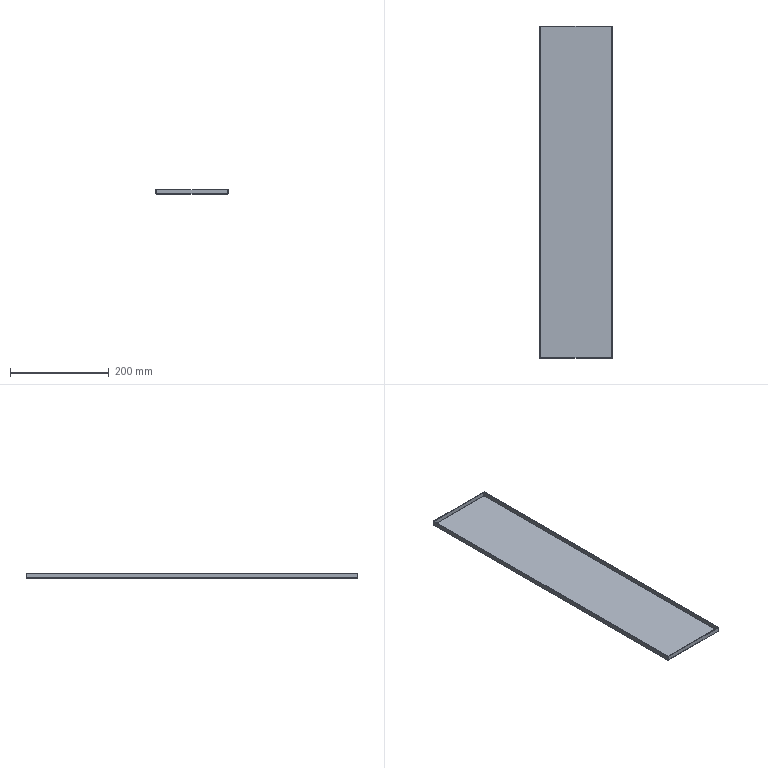Part | SolidWorks | features BaseBody 1 | 1 solid | 38 faces | box 146 x 672 x 10 mm | volume 166908 mm3 | plane 30 | cylinder 8 | commonest cylinder face diameters 0.4 x4 3.4 x4
STEP:
#1=CARTESIAN_POINT('',(1309.,40.5,426.7));
#2=VERTEX_POINT('',#1);
#3=CARTESIAN_POINT('',(1309.,40.7,426.5));
#4=VERTEX_POINT('',#3);
#5=CARTESIAN_POINT('',(1309.,40.7,426.7));
#6=DIRECTION('',(1.,0.,0.));
#7=DIRECTION('',(0.,1.,0.));
#8=AXIS2_PLACEMENT_3D('',#5,#6,#7);
#9=CIRCLE('',#8,0.2);
#10=EDGE_CURVE('',#2,#4,#9,.T.);
#11=ORIENTED_EDGE('',*,*,#10,.F.);
#12=CARTESIAN_POINT('',(1451.,40.5,426.7));
#13=VERTEX_POINT('',#12);
#14=CARTESIAN_POINT('',(1309.,40.5,426.7));
#15=DIRECTION('',(-1.,0.,0.));
#16=VECTOR('',#15,1000.);
#17=LINE('',#14,#16);
#18=EDGE_CURVE('',#13,#2,#17,.T.);
#19=ORIENTED_EDGE('',*,*,#18,.F.);
#20=CARTESIAN_POINT('',(1451.,40.7,426.5));
#21=VERTEX_POINT('',#20);
#22=CARTESIAN_POINT('',(1451.,40.7,426.7));
#23=DIRECTION('',(-1.,0.,0.));
#24=DIRECTION('',(0.,1.,0.));
#25=AXIS2_PLACEMENT_3D('',#22,#23,#24);
#26=CIRCLE('',#25,0.2);
#27=EDGE_CURVE('',#21,#13,#26,.T.);
#28=ORIENTED_EDGE('',*,*,#27,.F.);
#29=CARTESIAN_POINT('',(1309.,40.7,426.5));
#30=DIRECTION('',(1.,0.,0.));
#31=VECTOR('',#30,1000.);
#32=LINE('',#29,#31);
#33=EDGE_CURVE('',#4,#21,#32,.T.);
#34=ORIENTED_EDGE('',*,*,#33,.F.);
#35=EDGE_LOOP('',(#11,#19,#28,#34));
#36=FACE_OUTER_BOUND('',#35,.T.);
#37=CARTESIAN_POINT('',(613.969,40.7,426.7));
#38=DIRECTION('',(1.,0.,0.));
#39=DIRECTION('',(0.,1.,0.));
#40=AXIS2_PLACEMENT_3D('',#37,#38,#39);
#41=CYLINDRICAL_SURFACE('',#40,0.2);
#42=ADVANCED_FACE('',(#36),#41,.F.);
#43=CARTESIAN_POINT('',(1309.,39.,426.7));
#44=VERTEX_POINT('',#43);
#45=CARTESIAN_POINT('',(1309.,40.7,425.));
#46=VERTEX_POINT('',#45);
#47=CARTESIAN_POINT('',(1309.,40.7,426.7));
#48=DIRECTION('',(1.,0.,0.));
#49=DIRECTION('',(0.,1.,0.));
#50=AXIS2_PLACEMENT_3D('',#47,#48,#49);
#51=CIRCLE('',#50,1.7);
#52=EDGE_CURVE('',#44,#46,#51,.T.);
#53=ORIENTED_EDGE('',*,*,#52,.T.);
#54=CARTESIAN_POINT('',(1451.,40.7,425.));
#55=VERTEX_POINT('',#54);
#56=CARTESIAN_POINT('',(1309.,40.7,425.));
#57=DIRECTION('',(1.,0.,0.));
#58=VECTOR('',#57,1000.);
#59=LINE('',#56,#58);
#60=EDGE_CURVE('',#46,#55,#59,.T.);
#61=ORIENTED_EDGE('',*,*,#60,.T.);
#62=CARTESIAN_POINT('',(1451.,39.,426.7));
#63=VERTEX_POINT('',#62);
#64=CARTESIAN_POINT('',(1451.,40.7,426.7));
#65=DIRECTION('',(-1.,0.,0.));
#66=DIRECTION('',(0.,1.,0.));
#67=AXIS2_PLACEMENT_3D('',#64,#65,#66);
#68=CIRCLE('',#67,1.7);
#69=EDGE_CURVE('',#55,#63,#68,.T.);
#70=ORIENTED_EDGE('',*,*,#69,.T.);
#71=CARTESIAN_POINT('',(1309.,39.,426.7));
#72=DIRECTION('',(-1.,0.,0.));
#73=VECTOR('',#72,1000.);
#74=LINE('',#71,#73);
#75=EDGE_CURVE('',#63,#44,#74,.T.);
#76=ORIENTED_EDGE('',*,*,#75,.T.);
#77=EDGE_LOOP('',(#53,#61,#70,#76));
#78=FACE_OUTER_BOUND('',#77,.T.);
#79=CARTESIAN_POINT('',(613.969,40.7,426.7));
#80=DIRECTION('',(1.,0.,0.));
#81=DIRECTION('',(0.,1.,0.));
#82=AXIS2_PLACEMENT_3D('',#79,#80,#81);
#83=CYLINDRICAL_SURFACE('',#82,1.7);
#84=ADVANCED_FACE('',(#78),#83,.T.);
#85=CARTESIAN_POINT('',(1308.5,709.,426.7));
#86=VERTEX_POINT('',#85);
#87=CARTESIAN_POINT('',(1308.7,709.,426.5));
#88=VERTEX_POINT('',#87);
#89=CARTESIAN_POINT('',(1308.7,709.,426.7));
#90=DIRECTION('',(0.,-1.,0.));
#91=DIRECTION('',(0.,0.,-1.));
#92=AXIS2_PLACEMENT_3D('',#89,#90,#91);
#93=CIRCLE('',#92,0.2);
#94=EDGE_CURVE('',#86,#88,#93,.T.);
#95=ORIENTED_EDGE('',*,*,#94,.F.);
#96=CARTESIAN_POINT('',(1308.5,41.,426.7));
#97=VERTEX_POINT('',#96);
#98=CARTESIAN_POINT('',(1308.5,709.,426.7));
#99=DIRECTION('',(0.,1.,0.));
#100=VECTOR('',#99,1000.);
#101=LINE('',#98,#100);
#102=EDGE_CURVE('',#97,#86,#101,.T.);
#103=ORIENTED_EDGE('',*,*,#102,.F.);
#104=CARTESIAN_POINT('',(1308.7,41.,426.5));
#105=VERTEX_POINT('',#104);
#106=CARTESIAN_POINT('',(1308.7,41.,426.7));
#107=DIRECTION('',(0.,1.,0.));
#108=DIRECTION('',(0.,0.,-1.));
#109=AXIS2_PLACEMENT_3D('',#106,#107,#108);
#110=CIRCLE('',#109,0.2);
#111=EDGE_CURVE('',#105,#97,#110,.T.);
#112=ORIENTED_EDGE('',*,*,#111,.F.);
#113=CARTESIAN_POINT('',(1308.7,709.,426.5));
#114=DIRECTION('',(0.,-1.,0.));
#115=VECTOR('',#114,1000.);
#116=LINE('',#113,#115);
#117=EDGE_CURVE('',#88,#105,#116,.T.);
#118=ORIENTED_EDGE('',*,*,#117,.F.);
#119=EDGE_LOOP('',(#95,#103,#112,#118));
#120=FACE_OUTER_BOUND('',#119,.T.);
#121=CARTESIAN_POINT('',(1308.7,1405.634,426.7));
#122=DIRECTION('',(0.,-1.,0.));
#123=DIRECTION('',(0.,0.,-1.));
#124=AXIS2_PLACEMENT_3D('',#121,#122,#123);
#125=CYLINDRICAL_SURFACE('',#124,0.2);
#126=ADVANCED_FACE('',(#120),#125,.F.);
#127=CARTESIAN_POINT('',(1307.,709.,426.7));
#128=VERTEX_POINT('',#127);
#129=CARTESIAN_POINT('',(1308.7,709.,425.));
#130=VERTEX_POINT('',#129);
#131=CARTESIAN_POINT('',(1308.7,709.,426.7));
#132=DIRECTION('',(0.,-1.,0.));
#133=DIRECTION('',(0.,0.,-1.));
#134=AXIS2_PLACEMENT_3D('',#131,#132,#133);
#135=CIRCLE('',#134,1.7);
#136=EDGE_CURVE('',#128,#130,#135,.T.);
#137=ORIENTED_EDGE('',*,*,#136,.T.);
#138=CARTESIAN_POINT('',(1308.7,41.,425.));
#139=VERTEX_POINT('',#138);
#140=CARTESIAN_POINT('',(1308.7,709.,425.));
#141=DIRECTION('',(0.,-1.,0.));
#142=VECTOR('',#141,1000.);
#143=LINE('',#140,#142);
#144=EDGE_CURVE('',#130,#139,#143,.T.);
#145=ORIENTED_EDGE('',*,*,#144,.T.);
#146=CARTESIAN_POINT('',(1307.,41.,426.7));
#147=VERTEX_POINT('',#146);
#148=CARTESIAN_POINT('',(1308.7,41.,426.7));
#149=DIRECTION('',(0.,1.,0.));
#150=DIRECTION('',(0.,0.,-1.));
#151=AXIS2_PLACEMENT_3D('',#148,#149,#150);
#152=CIRCLE('',#151,1.7);
#153=EDGE_CURVE('',#139,#147,#152,.T.);
#154=ORIENTED_EDGE('',*,*,#153,.T.);
#155=CARTESIAN_POINT('',(1307.,709.,426.7));
#156=DIRECTION('',(0.,1.,0.));
#157=VECTOR('',#156,1000.);
#158=LINE('',#155,#157);
#159=EDGE_CURVE('',#147,#128,#158,.T.);
#160=ORIENTED_EDGE('',*,*,#159,.T.);
#161=EDGE_LOOP('',(#137,#145,#154,#160));
#162=FACE_OUTER_BOUND('',#161,.T.);
#163=CARTESIAN_POINT('',(1308.7,1405.634,426.7));
#164=DIRECTION('',(0.,-1.,0.));
#165=DIRECTION('',(0.,0.,-1.));
#166=AXIS2_PLACEMENT_3D('',#163,#164,#165);
#167=CYLINDRICAL_SURFACE('',#166,1.7);
#168=ADVANCED_FACE('',(#162),#167,.T.);
#169=CARTESIAN_POINT('',(1451.,709.5,426.7));
#170=VERTEX_POINT('',#169);
#171=CARTESIAN_POINT('',(1451.,709.3,426.5));
#172=VERTEX_POINT('',#171);
#173=CARTESIAN_POINT('',(1451.,709.3,426.7));
#174=DIRECTION('',(-1.,0.,0.));
#175=DIRECTION('',(0.,0.,1.));
#176=AXIS2_PLACEMENT_3D('',#173,#174,#175);
#177=CIRCLE('',#176,0.2);
#178=EDGE_CURVE('',#170,#172,#177,.T.);
#179=ORIENTED_EDGE('',*,*,#178,.F.);
#180=CARTESIAN_POINT('',(1309.,709.5,426.7));
#181=VERTEX_POINT('',#180);
#182=CARTESIAN_POINT('',(1451.,709.5,426.7));
#183=DIRECTION('',(1.,0.,0.));
#184=VECTOR('',#183,1000.);
#185=LINE('',#182,#184);
#186=EDGE_CURVE('',#181,#170,#185,.T.);
#187=ORIENTED_EDGE('',*,*,#186,.F.);
#188=CARTESIAN_POINT('',(1309.,709.3,426.5));
#189=VERTEX_POINT('',#188);
#190=CARTESIAN_POINT('',(1309.,709.3,426.7));
#191=DIRECTION('',(1.,0.,0.));
#192=DIRECTION('',(0.,0.,1.));
#193=AXIS2_PLACEMENT_3D('',#190,#191,#192);
#194=CIRCLE('',#193,0.2);
#195=EDGE_CURVE('',#189,#181,#194,.T.);
#196=ORIENTED_EDGE('',*,*,#195,.F.);
#197=CARTESIAN_POINT('',(1451.,709.3,426.5));
#198=DIRECTION('',(-1.,0.,0.));
#199=VECTOR('',#198,1000.);
#200=LINE('',#197,#199);
#201=EDGE_CURVE('',#172,#189,#200,.T.);
#202=ORIENTED_EDGE('',*,*,#201,.F.);
#203=EDGE_LOOP('',(#179,#187,#196,#202));
#204=FACE_OUTER_BOUND('',#203,.T.);
#205=CARTESIAN_POINT('',(2154.902,709.3,426.7));
#206=DIRECTION('',(-1.,0.,0.));
#207=DIRECTION('',(0.,0.,1.));
#208=AXIS2_PLACEMENT_3D('',#205,#206,#207);
#209=CYLINDRICAL_SURFACE('',#208,0.2);
#210=ADVANCED_FACE('',(#204),#209,.F.);
#211=CARTESIAN_POINT('',(1451.,711.,426.7));
#212=VERTEX_POINT('',#211);
#213=CARTESIAN_POINT('',(1451.,709.3,425.));
#214=VERTEX_POINT('',#213);
#215=CARTESIAN_POINT('',(1451.,709.3,426.7));
#216=DIRECTION('',(-1.,0.,0.));
#217=DIRECTION('',(0.,0.,1.));
#218=AXIS2_PLACEMENT_3D('',#215,#216,#217);
#219=CIRCLE('',#218,1.7);
#220=EDGE_CURVE('',#212,#214,#219,.T.);
#221=ORIENTED_EDGE('',*,*,#220,.T.);
#222=CARTESIAN_POINT('',(1309.,709.3,425.));
#223=VERTEX_POINT('',#222);
#224=CARTESIAN_POINT('',(1451.,709.3,425.));
#225=DIRECTION('',(-1.,0.,0.));
#226=VECTOR('',#225,1000.);
#227=LINE('',#224,#226);
#228=EDGE_CURVE('',#214,#223,#227,.T.);
#229=ORIENTED_EDGE('',*,*,#228,.T.);
#230=CARTESIAN_POINT('',(1309.,711.,426.7));
#231=VERTEX_POINT('',#230);
#232=CARTESIAN_POINT('',(1309.,709.3,426.7));
#233=DIRECTION('',(1.,0.,0.));
#234=DIRECTION('',(0.,0.,1.));
#235=AXIS2_PLACEMENT_3D('',#232,#233,#234);
#236=CIRCLE('',#235,1.7);
#237=EDGE_CURVE('',#223,#231,#236,.T.);
#238=ORIENTED_EDGE('',*,*,#237,.T.);
#239=CARTESIAN_POINT('',(1451.,711.,426.7));
#240=DIRECTION('',(1.,0.,0.));
#241=VECTOR('',#240,1000.);
#242=LINE('',#239,#241);
#243=EDGE_CURVE('',#231,#212,#242,.T.);
#244=ORIENTED_EDGE('',*,*,#243,.T.);
#245=EDGE_LOOP('',(#221,#229,#238,#244));
#246=FACE_OUTER_BOUND('',#245,.T.);
#247=CARTESIAN_POINT('',(2154.902,709.3,426.7));
#248=DIRECTION('',(-1.,0.,0.));
#249=DIRECTION('',(0.,0.,1.));
#250=AXIS2_PLACEMENT_3D('',#247,#248,#249);
#251=CYLINDRICAL_SURFACE('',#250,1.7);
#252=ADVANCED_FACE('',(#246),#251,.T.);
#253=CARTESIAN_POINT('',(1451.5,41.,426.7));
#254=VERTEX_POINT('',#253);
#255=CARTESIAN_POINT('',(1451.3,41.,426.5));
#256=VERTEX_POINT('',#255);
#257=CARTESIAN_POINT('',(1451.3,41.,426.7));
#258=DIRECTION('',(0.,1.,0.));
#259=DIRECTION('',(0.,0.,1.));
#260=AXIS2_PLACEMENT_3D('',#257,#258,#259);
#261=CIRCLE('',#260,0.2);
#262=EDGE_CURVE('',#254,#256,#261,.T.);
#263=ORIENTED_EDGE('',*,*,#262,.F.);
#264=CARTESIAN_POINT('',(1451.5,709.,426.7));
#265=VERTEX_POINT('',#264);
#266=CARTESIAN_POINT('',(1451.5,41.,426.7));
#267=DIRECTION('',(0.,-1.,0.));
#268=VECTOR('',#267,1000.);
#269=LINE('',#266,#268);
#270=EDGE_CURVE('',#265,#254,#269,.T.);
#271=ORIENTED_EDGE('',*,*,#270,.F.);
#272=CARTESIAN_POINT('',(1451.3,709.,426.5));
#273=VERTEX_POINT('',#272);
#274=CARTESIAN_POINT('',(1451.3,709.,426.7));
#275=DIRECTION('',(0.,-1.,0.));
#276=DIRECTION('',(0.,0.,1.));
#277=AXIS2_PLACEMENT_3D('',#274,#275,#276);
#278=CIRCLE('',#277,0.2);
#279=EDGE_CURVE('',#273,#265,#278,.T.);
#280=ORIENTED_EDGE('',*,*,#279,.F.);
#281=CARTESIAN_POINT('',(1451.3,41.,426.5));
#282=DIRECTION('',(0.,1.,0.));
#283=VECTOR('',#282,1000.);
#284=LINE('',#281,#283);
#285=EDGE_CURVE('',#256,#273,#284,.T.);
#286=ORIENTED_EDGE('',*,*,#285,.F.);
#287=EDGE_LOOP('',(#263,#271,#280,#286));
#288=FACE_OUTER_BOUND('',#287,.T.);
#289=CARTESIAN_POINT('',(1451.3,-664.495,426.7));
#290=DIRECTION('',(0.,1.,0.));
#291=DIRECTION('',(0.,0.,1.));
#292=AXIS2_PLACEMENT_3D('',#289,#290,#291);
#293=CYLINDRICAL_SURFACE('',#292,0.2);
#294=ADVANCED_FACE('',(#288),#293,.F.);
#295=CARTESIAN_POINT('',(1453.,41.,426.7));
#296=VERTEX_POINT('',#295);
#297=CARTESIAN_POINT('',(1451.3,41.,425.));
#298=VERTEX_POINT('',#297);
#299=CARTESIAN_POINT('',(1451.3,41.,426.7));
#300=DIRECTION('',(0.,1.,0.));
#301=DIRECTION('',(0.,0.,1.));
#302=AXIS2_PLACEMENT_3D('',#299,#300,#301);
#303=CIRCLE('',#302,1.7);
#304=EDGE_CURVE('',#296,#298,#303,.T.);
#305=ORIENTED_EDGE('',*,*,#304,.T.);
#306=CARTESIAN_POINT('',(1451.3,709.,425.));
#307=VERTEX_POINT('',#306);
#308=CARTESIAN_POINT('',(1451.3,41.,425.));
#309=DIRECTION('',(0.,1.,0.));
#310=VECTOR('',#309,1000.);
#311=LINE('',#308,#310);
#312=EDGE_CURVE('',#298,#307,#311,.T.);
#313=ORIENTED_EDGE('',*,*,#312,.T.);
#314=CARTESIAN_POINT('',(1453.,709.,426.7));
#315=VERTEX_POINT('',#314);
#316=CARTESIAN_POINT('',(1451.3,709.,426.7));
#317=DIRECTION('',(0.,-1.,0.));
#318=DIRECTION('',(0.,0.,1.));
#319=AXIS2_PLACEMENT_3D('',#316,#317,#318);
#320=CIRCLE('',#319,1.7);
#321=EDGE_CURVE('',#307,#315,#320,.T.);
#322=ORIENTED_EDGE('',*,*,#321,.T.);
#323=CARTESIAN_POINT('',(1453.,41.,426.7));
#324=DIRECTION('',(0.,-1.,0.));
#325=VECTOR('',#324,1000.);
#326=LINE('',#323,#325);
#327=EDGE_CURVE('',#315,#296,#326,.T.);
#328=ORIENTED_EDGE('',*,*,#327,.T.);
#329=EDGE_LOOP('',(#305,#313,#322,#328));
#330=FACE_OUTER_BOUND('',#329,.T.);
#331=CARTESIAN_POINT('',(1451.3,-664.495,426.7));
#332=DIRECTION('',(0.,1.,0.));
#333=DIRECTION('',(0.,0.,1.));
#334=AXIS2_PLACEMENT_3D('',#331,#332,#333);
#335=CYLINDRICAL_SURFACE('',#334,1.7);
#336=ADVANCED_FACE('',(#330),#335,.T.);
#337=CARTESIAN_POINT('',(1451.,41.,426.5));
#338=VERTEX_POINT('',#337);
#339=CARTESIAN_POINT('',(0.,41.,426.5));
#340=DIRECTION('',(1.,0.,0.));
#341=VECTOR('',#340,1000.);
#342=LINE('',#339,#341);
#343=EDGE_CURVE('',#338,#256,#342,.T.);
#344=ORIENTED_EDGE('',*,*,#343,.T.);
#345=ORIENTED_EDGE('',*,*,#285,.T.);
#346=CARTESIAN_POINT('',(1451.,709.,426.5));
#347=VERTEX_POINT('',#346);
#348=CARTESIAN_POINT('',(0.,709.,426.5));
#349=DIRECTION('',(-1.,0.,0.));
#350=VECTOR('',#349,1000.);
#351=LINE('',#348,#350);
#352=EDGE_CURVE('',#273,#347,#351,.T.);
#353=ORIENTED_EDGE('',*,*,#352,.T.);
#354=CARTESIAN_POINT('',(1451.,0.,426.5));
#355=DIRECTION('',(0.,1.,0.));
#356=VECTOR('',#355,1000.);
#357=LINE('',#354,#356);
#358=EDGE_CURVE('',#347,#172,#357,.T.);
#359=ORIENTED_EDGE('',*,*,#358,.T.);
#360=ORIENTED_EDGE('',*,*,#201,.T.);
#361=CARTESIAN_POINT('',(1309.,709.,426.5));
#362=VERTEX_POINT('',#361);
#363=CARTESIAN_POINT('',(1309.,0.,426.5));
#364=DIRECTION('',(0.,-1.,0.));
#365=VECTOR('',#364,1000.);
#366=LINE('',#363,#365);
#367=EDGE_CURVE('',#189,#362,#366,.T.);
#368=ORIENTED_EDGE('',*,*,#367,.T.);
#369=CARTESIAN_POINT('',(0.,709.,426.5));
#370=DIRECTION('',(-1.,0.,0.));
#371=VECTOR('',#370,1000.);
#372=LINE('',#369,#371);
#373=EDGE_CURVE('',#362,#88,#372,.T.);
#374=ORIENTED_EDGE('',*,*,#373,.T.);
#375=ORIENTED_EDGE('',*,*,#117,.T.);
#376=CARTESIAN_POINT('',(1309.,41.,426.5));
#377=VERTEX_POINT('',#376);
#378=CARTESIAN_POINT('',(0.,41.,426.5));
#379=DIRECTION('',(1.,0.,0.));
#380=VECTOR('',#379,1000.);
#381=LINE('',#378,#380);
#382=EDGE_CURVE('',#105,#377,#381,.T.);
#383=ORIENTED_EDGE('',*,*,#382,.T.);
#384=CARTESIAN_POINT('',(1309.,0.,426.5));
#385=DIRECTION('',(0.,-1.,0.));
#386=VECTOR('',#385,1000.);
#387=LINE('',#384,#386);
#388=EDGE_CURVE('',#377,#4,#387,.T.);
#389=ORIENTED_EDGE('',*,*,#388,.T.);
#390=ORIENTED_EDGE('',*,*,#33,.T.);
#391=CARTESIAN_POINT('',(1451.,0.,426.5));
#392=DIRECTION('',(0.,1.,0.));
#393=VECTOR('',#392,1000.);
#394=LINE('',#391,#393);
#395=EDGE_CURVE('',#21,#338,#394,.T.);
#396=ORIENTED_EDGE('',*,*,#395,.T.);
#397=EDGE_LOOP('',(#344,#345,#353,#359,#360,#368,#374,#375,#383,#389,#390,#396));
#398=FACE_OUTER_BOUND('',#397,.T.);
#399=CARTESIAN_POINT('',(0.,0.,426.5));
#400=DIRECTION('',(0.,0.,1.));
#401=DIRECTION('',(1.,0.,0.));
#402=AXIS2_PLACEMENT_3D('',#399,#400,#401);
#403=PLANE('',#402);
#404=ADVANCED_FACE('',(#398),#403,.T.);
#405=ORIENTED_EDGE('',*,*,#382,.F.);
#406=ORIENTED_EDGE('',*,*,#111,.T.);
#407=CARTESIAN_POINT('',(2652.603,41.,426.7));
#408=DIRECTION('',(-1.,0.,0.));
#409=VECTOR('',#408,1000.);
#410=LINE('',#407,#409);
#411=EDGE_CURVE('',#97,#147,#410,.T.);
#412=ORIENTED_EDGE('',*,*,#411,.T.);
#413=ORIENTED_EDGE('',*,*,#153,.F.);
#414=CARTESIAN_POINT('',(1309.,41.,425.));
#415=VERTEX_POINT('',#414);
#416=CARTESIAN_POINT('',(0.,41.,425.));
#417=DIRECTION('',(1.,0.,0.));
#418=VECTOR('',#417,1000.);
#419=LINE('',#416,#418);
#420=EDGE_CURVE('',#139,#415,#419,.T.);
#421=ORIENTED_EDGE('',*,*,#420,.T.);
#422=CARTESIAN_POINT('',(1309.,41.,1793.776));
#423=DIRECTION('',(0.,0.,-1.));
#424=VECTOR('',#423,1000.);
#425=LINE('',#422,#424);
#426=EDGE_CURVE('',#377,#415,#425,.T.);
#427=ORIENTED_EDGE('',*,*,#426,.F.);
#428=EDGE_LOOP('',(#405,#406,#412,#413,#421,#427));
#429=FACE_OUTER_BOUND('',#428,.T.);
#430=CARTESIAN_POINT('',(0.,41.,1793.776));
#431=DIRECTION('',(0.,1.,0.));
#432=DIRECTION('',(1.,0.,0.));
#433=AXIS2_PLACEMENT_3D('',#430,#431,#432);
#434=PLANE('',#433);
#435=ADVANCED_FACE('',(#429),#434,.F.);
#436=CARTESIAN_POINT('',(1309.,709.,425.));
#437=VERTEX_POINT('',#436);
#438=CARTESIAN_POINT('',(1309.,709.,1793.776));
#439=DIRECTION('',(0.,0.,-1.));
#440=VECTOR('',#439,1000.);
#441=LINE('',#438,#440);
#442=EDGE_CURVE('',#362,#437,#441,.T.);
#443=ORIENTED_EDGE('',*,*,#442,.T.);
#444=CARTESIAN_POINT('',(0.,709.,425.));
#445=DIRECTION('',(-1.,0.,0.));
#446=VECTOR('',#445,1000.);
#447=LINE('',#444,#446);
#448=EDGE_CURVE('',#437,#130,#447,.T.);
#449=ORIENTED_EDGE('',*,*,#448,.T.);
#450=ORIENTED_EDGE('',*,*,#136,.F.);
#451=CARTESIAN_POINT('',(2652.603,709.,426.7));
#452=DIRECTION('',(-1.,0.,0.));
#453=VECTOR('',#452,1000.);
#454=LINE('',#451,#453);
#455=EDGE_CURVE('',#86,#128,#454,.T.);
#456=ORIENTED_EDGE('',*,*,#455,.F.);
#457=ORIENTED_EDGE('',*,*,#94,.T.);
#458=ORIENTED_EDGE('',*,*,#373,.F.);
#459=EDGE_LOOP('',(#443,#449,#450,#456,#457,#458));
#460=FACE_OUTER_BOUND('',#459,.T.);
#461=CARTESIAN_POINT('',(0.,709.,1793.776));
#462=DIRECTION('',(0.,-1.,0.));
#463=DIRECTION('',(0.,0.,-1.));
#464=AXIS2_PLACEMENT_3D('',#461,#462,#463);
#465=PLANE('',#464);
#466=ADVANCED_FACE('',(#460),#465,.F.);
#467=ORIENTED_EDGE('',*,*,#352,.F.);
#468=ORIENTED_EDGE('',*,*,#279,.T.);
#469=CARTESIAN_POINT('',(107.397,709.,426.7));
#470=DIRECTION('',(1.,0.,0.));
#471=VECTOR('',#470,1000.);
#472=LINE('',#469,#471);
#473=EDGE_CURVE('',#265,#315,#472,.T.);
#474=ORIENTED_EDGE('',*,*,#473,.T.);
#475=ORIENTED_EDGE('',*,*,#321,.F.);
#476=CARTESIAN_POINT('',(1451.,709.,425.));
#477=VERTEX_POINT('',#476);
#478=CARTESIAN_POINT('',(0.,709.,425.));
#479=DIRECTION('',(-1.,0.,0.));
#480=VECTOR('',#479,1000.);
#481=LINE('',#478,#480);
#482=EDGE_CURVE('',#307,#477,#481,.T.);
#483=ORIENTED_EDGE('',*,*,#482,.T.);
#484=CARTESIAN_POINT('',(1451.,709.,1793.776));
#485=DIRECTION('',(0.,0.,-1.));
#486=VECTOR('',#485,1000.);
#487=LINE('',#484,#486);
#488=EDGE_CURVE('',#347,#477,#487,.T.);
#489=ORIENTED_EDGE('',*,*,#488,.F.);
#490=EDGE_LOOP('',(#467,#468,#474,#475,#483,#489));
#491=FACE_OUTER_BOUND('',#490,.T.);
#492=CARTESIAN_POINT('',(0.,709.,1793.776));
#493=DIRECTION('',(0.,-1.,0.));
#494=DIRECTION('',(0.,0.,-1.));
#495=AXIS2_PLACEMENT_3D('',#492,#493,#494);
#496=PLANE('',#495);
#497=ADVANCED_FACE('',(#491),#496,.F.);
#498=CARTESIAN_POINT('',(1451.,41.,425.));
#499=VERTEX_POINT('',#498);
#500=CARTESIAN_POINT('',(1451.,41.,1793.776));
#501=DIRECTION('',(0.,0.,-1.));
#502=VECTOR('',#501,1000.);
#503=LINE('',#500,#502);
#504=EDGE_CURVE('',#338,#499,#503,.T.);
#505=ORIENTED_EDGE('',*,*,#504,.T.);
#506=CARTESIAN_POINT('',(0.,41.,425.));
#507=DIRECTION('',(1.,0.,0.));
#508=VECTOR('',#507,1000.);
#509=LINE('',#506,#508);
#510=EDGE_CURVE('',#499,#298,#509,.T.);
#511=ORIENTED_EDGE('',*,*,#510,.T.);
#512=ORIENTED_EDGE('',*,*,#304,.F.);
#513=CARTESIAN_POINT('',(107.397,41.,426.7));
#514=DIRECTION('',(1.,0.,0.));
#515=VECTOR('',#514,1000.);
#516=LINE('',#513,#515);
#517=EDGE_CURVE('',#254,#296,#516,.T.);
#518=ORIENTED_EDGE('',*,*,#517,.F.);
#519=ORIENTED_EDGE('',*,*,#262,.T.);
#520=ORIENTED_EDGE('',*,*,#343,.F.);
#521=EDGE_LOOP('',(#505,#511,#512,#518,#519,#520));
#522=FACE_OUTER_BOUND('',#521,.T.);
#523=CARTESIAN_POINT('',(0.,41.,1793.776));
#524=DIRECTION('',(0.,1.,0.));
#525=DIRECTION('',(1.,0.,0.));
#526=AXIS2_PLACEMENT_3D('',#523,#524,#525);
#527=PLANE('',#526);
#528=ADVANCED_FACE('',(#522),#527,.F.);
#529=ORIENTED_EDGE('',*,*,#312,.F.);
#530=ORIENTED_EDGE('',*,*,#510,.F.);
#531=CARTESIAN_POINT('',(1451.,0.,425.));
#532=DIRECTION('',(0.,1.,0.));
#533=VECTOR('',#532,1000.);
#534=LINE('',#531,#533);
#535=EDGE_CURVE('',#55,#499,#534,.T.);
#536=ORIENTED_EDGE('',*,*,#535,.F.);
#537=ORIENTED_EDGE('',*,*,#60,.F.);
#538=CARTESIAN_POINT('',(1309.,0.,425.));
#539=DIRECTION('',(0.,-1.,0.));
#540=VECTOR('',#539,1000.);
#541=LINE('',#538,#540);
#542=EDGE_CURVE('',#415,#46,#541,.T.);
#543=ORIENTED_EDGE('',*,*,#542,.F.);
#544=ORIENTED_EDGE('',*,*,#420,.F.);
#545=ORIENTED_EDGE('',*,*,#144,.F.);
#546=ORIENTED_EDGE('',*,*,#448,.F.);
#547=CARTESIAN_POINT('',(1309.,0.,425.));
#548=DIRECTION('',(0.,-1.,0.));
#549=VECTOR('',#548,1000.);
#550=LINE('',#547,#549);
#551=EDGE_CURVE('',#223,#437,#550,.T.);
#552=ORIENTED_EDGE('',*,*,#551,.F.);
#553=ORIENTED_EDGE('',*,*,#228,.F.);
#554=CARTESIAN_POINT('',(1451.,0.,425.));
#555=DIRECTION('',(0.,1.,0.));
#556=VECTOR('',#555,1000.);
#557=LINE('',#554,#556);
#558=EDGE_CURVE('',#477,#214,#557,.T.);
#559=ORIENTED_EDGE('',*,*,#558,.F.);
#560=ORIENTED_EDGE('',*,*,#482,.F.);
#561=EDGE_LOOP('',(#529,#530,#536,#537,#543,#544,#545,#546,#552,#553,#559,#560));
#562=FACE_OUTER_BOUND('',#561,.T.);
#563=CARTESIAN_POINT('',(0.,0.,425.));
#564=DIRECTION('',(0.,0.,1.));
#565=DIRECTION('',(1.,0.,0.));
#566=AXIS2_PLACEMENT_3D('',#563,#564,#565);
#567=PLANE('',#566);
#568=ADVANCED_FACE('',(#562),#567,.F.);
#569=CARTESIAN_POINT('',(1451.5,39.,435.));
#570=VERTEX_POINT('',#569);
#571=CARTESIAN_POINT('',(1451.5,711.,435.));
#572=VERTEX_POINT('',#571);
#573=CARTESIAN_POINT('',(1451.5,40.5,435.));
#574=DIRECTION('',(0.,1.,0.));
#575=VECTOR('',#574,1000.);
#576=LINE('',#573,#575);
#577=EDGE_CURVE('',#570,#572,#576,.T.);
#578=ORIENTED_EDGE('',*,*,#577,.T.);
#579=CARTESIAN_POINT('',(1451.5,711.,426.7));
#580=VERTEX_POINT('',#579);
#581=CARTESIAN_POINT('',(1451.5,711.,-259.113));
#582=DIRECTION('',(0.,0.,-1.));
#583=VECTOR('',#582,1000.);
#584=LINE('',#581,#583);
#585=EDGE_CURVE('',#572,#580,#584,.T.);
#586=ORIENTED_EDGE('',*,*,#585,.T.);
#587=CARTESIAN_POINT('',(1451.5,711.002,426.7));
#588=DIRECTION('',(0.,-1.,0.));
#589=VECTOR('',#588,1000.);
#590=LINE('',#587,#589);
#591=EDGE_CURVE('',#580,#265,#590,.T.);
#592=ORIENTED_EDGE('',*,*,#591,.T.);
#593=ORIENTED_EDGE('',*,*,#270,.T.);
#594=CARTESIAN_POINT('',(1451.5,39.,426.7));
#595=VERTEX_POINT('',#594);
#596=CARTESIAN_POINT('',(1451.5,38.998,426.7));
#597=DIRECTION('',(0.,1.,0.));
#598=VECTOR('',#597,1000.);
#599=LINE('',#596,#598);
#600=EDGE_CURVE('',#595,#254,#599,.T.);
#601=ORIENTED_EDGE('',*,*,#600,.F.);
#602=CARTESIAN_POINT('',(1451.5,39.,-259.113));
#603=DIRECTION('',(0.,0.,1.));
#604=VECTOR('',#603,1000.);
#605=LINE('',#602,#604);
#606=EDGE_CURVE('',#595,#570,#605,.T.);
#607=ORIENTED_EDGE('',*,*,#606,.T.);
#608=EDGE_LOOP('',(#578,#586,#592,#593,#601,#607));
#609=FACE_OUTER_BOUND('',#608,.T.);
#610=CARTESIAN_POINT('',(1451.5,40.5,-259.113));
#611=DIRECTION('',(1.,0.,0.));
#612=DIRECTION('',(0.,1.,0.));
#613=AXIS2_PLACEMENT_3D('',#610,#611,#612);
#614=PLANE('',#613);
#615=ADVANCED_FACE('',(#609),#614,.F.);
#616=CARTESIAN_POINT('',(1453.,711.,426.7));
#617=VERTEX_POINT('',#616);
#618=CARTESIAN_POINT('',(1453.,711.002,426.7));
#619=DIRECTION('',(0.,-1.,0.));
#620=VECTOR('',#619,1000.);
#621=LINE('',#618,#620);
#622=EDGE_CURVE('',#617,#315,#621,.T.);
#623=ORIENTED_EDGE('',*,*,#622,.T.);
#624=ORIENTED_EDGE('',*,*,#473,.F.);
#625=ORIENTED_EDGE('',*,*,#591,.F.);
#626=CARTESIAN_POINT('',(107.397,711.,426.7));
#627=DIRECTION('',(1.,0.,0.));
#628=VECTOR('',#627,1000.);
#629=LINE('',#626,#628);
#630=EDGE_CURVE('',#580,#617,#629,.T.);
#631=ORIENTED_EDGE('',*,*,#630,.T.);
#632=EDGE_LOOP('',(#623,#624,#625,#631));
#633=FACE_OUTER_BOUND('',#632,.T.);
#634=CARTESIAN_POINT('',(107.397,711.002,426.7));
#635=DIRECTION('',(0.,0.,1.));
#636=DIRECTION('',(1.,0.,0.));
#637=AXIS2_PLACEMENT_3D('',#634,#635,#636);
#638=PLANE('',#637);
#639=ADVANCED_FACE('',(#633),#638,.F.);
#640=ORIENTED_EDGE('',*,*,#327,.F.);
#641=ORIENTED_EDGE('',*,*,#622,.F.);
#642=CARTESIAN_POINT('',(1453.,711.,435.));
#643=VERTEX_POINT('',#642);
#644=CARTESIAN_POINT('',(1453.,711.,-259.113));
#645=DIRECTION('',(0.,0.,1.));
#646=VECTOR('',#645,1000.);
#647=LINE('',#644,#646);
#648=EDGE_CURVE('',#617,#643,#647,.T.);
#649=ORIENTED_EDGE('',*,*,#648,.T.);
#650=CARTESIAN_POINT('',(1453.,39.,435.));
#651=VERTEX_POINT('',#650);
#652=CARTESIAN_POINT('',(1453.,39.,435.));
#653=DIRECTION('',(0.,-1.,0.));
#654=VECTOR('',#653,1000.);
#655=LINE('',#652,#654);
#656=EDGE_CURVE('',#643,#651,#655,.T.);
#657=ORIENTED_EDGE('',*,*,#656,.T.);
#658=CARTESIAN_POINT('',(1453.,39.,426.7));
#659=VERTEX_POINT('',#658);
#660=CARTESIAN_POINT('',(1453.,39.,423.672));
#661=DIRECTION('',(0.,0.,1.));
#662=VECTOR('',#661,1000.);
#663=LINE('',#660,#662);
#664=EDGE_CURVE('',#659,#651,#663,.T.);
#665=ORIENTED_EDGE('',*,*,#664,.F.);
#666=CARTESIAN_POINT('',(1453.,38.998,426.7));
#667=DIRECTION('',(0.,1.,0.));
#668=VECTOR('',#667,1000.);
#669=LINE('',#666,#668);
#670=EDGE_CURVE('',#659,#296,#669,.T.);
#671=ORIENTED_EDGE('',*,*,#670,.T.);
#672=EDGE_LOOP('',(#640,#641,#649,#657,#665,#671));
#673=FACE_OUTER_BOUND('',#672,.T.);
#674=CARTESIAN_POINT('',(1453.,39.,435.));
#675=DIRECTION('',(1.,0.,0.));
#676=DIRECTION('',(0.,1.,0.));
#677=AXIS2_PLACEMENT_3D('',#674,#675,#676);
#678=PLANE('',#677);
#679=ADVANCED_FACE('',(#673),#678,.T.);
#680=ORIENTED_EDGE('',*,*,#517,.T.);
#681=ORIENTED_EDGE('',*,*,#670,.F.);
#682=CARTESIAN_POINT('',(107.397,39.,426.7));
#683=DIRECTION('',(1.,0.,0.));
#684=VECTOR('',#683,1000.);
#685=LINE('',#682,#684);
#686=EDGE_CURVE('',#595,#659,#685,.T.);
#687=ORIENTED_EDGE('',*,*,#686,.F.);
#688=ORIENTED_EDGE('',*,*,#600,.T.);
#689=EDGE_LOOP('',(#680,#681,#687,#688));
#690=FACE_OUTER_BOUND('',#689,.T.);
#691=CARTESIAN_POINT('',(107.397,38.998,426.7));
#692=DIRECTION('',(0.,0.,-1.));
#693=DIRECTION('',(0.,-1.,0.));
#694=AXIS2_PLACEMENT_3D('',#691,#692,#693);
#695=PLANE('',#694);
#696=ADVANCED_FACE('',(#690),#695,.T.);
#697=ORIENTED_EDGE('',*,*,#664,.T.);
#698=CARTESIAN_POINT('',(107.397,39.,435.));
#699=DIRECTION('',(1.,0.,0.));
#700=VECTOR('',#699,1000.);
#701=LINE('',#698,#700);
#702=EDGE_CURVE('',#570,#651,#701,.T.);
#703=ORIENTED_EDGE('',*,*,#702,.F.);
#704=ORIENTED_EDGE('',*,*,#606,.F.);
#705=ORIENTED_EDGE('',*,*,#686,.T.);
#706=EDGE_LOOP('',(#697,#703,#704,#705));
#707=FACE_OUTER_BOUND('',#706,.T.);
#708=CARTESIAN_POINT('',(107.397,39.,-259.113));
#709=DIRECTION('',(0.,1.,0.));
#710=DIRECTION('',(0.,0.,-1.));
#711=AXIS2_PLACEMENT_3D('',#708,#709,#710);
#712=PLANE('',#711);
#713=ADVANCED_FACE('',(#707),#712,.F.);
#714=ORIENTED_EDGE('',*,*,#648,.F.);
#715=ORIENTED_EDGE('',*,*,#630,.F.);
#716=ORIENTED_EDGE('',*,*,#585,.F.);
#717=CARTESIAN_POINT('',(107.397,711.,435.));
#718=DIRECTION('',(1.,0.,0.));
#719=VECTOR('',#718,1000.);
#720=LINE('',#717,#719);
#721=EDGE_CURVE('',#572,#643,#720,.T.);
#722=ORIENTED_EDGE('',*,*,#721,.T.);
#723=EDGE_LOOP('',(#714,#715,#716,#722));
#724=FACE_OUTER_BOUND('',#723,.T.);
#725=CARTESIAN_POINT('',(107.397,711.,-259.113));
#726=DIRECTION('',(0.,-1.,0.));
#727=DIRECTION('',(0.,0.,-1.));
#728=AXIS2_PLACEMENT_3D('',#725,#726,#727);
#729=PLANE('',#728);
#730=ADVANCED_FACE('',(#724),#729,.F.);
#731=ORIENTED_EDGE('',*,*,#656,.F.);
#732=ORIENTED_EDGE('',*,*,#721,.F.);
#733=ORIENTED_EDGE('',*,*,#577,.F.);
#734=ORIENTED_EDGE('',*,*,#702,.T.);
#735=EDGE_LOOP('',(#731,#732,#733,#734));
#736=FACE_OUTER_BOUND('',#735,.T.);
#737=CARTESIAN_POINT('',(107.397,40.5,435.));
#738=DIRECTION('',(0.,0.,-1.));
#739=DIRECTION('',(0.,-1.,0.));
#740=AXIS2_PLACEMENT_3D('',#737,#738,#739);
#741=PLANE('',#740);
#742=ADVANCED_FACE('',(#736),#741,.F.);
#743=CARTESIAN_POINT('',(1309.,709.5,435.));
#744=VERTEX_POINT('',#743);
#745=CARTESIAN_POINT('',(1309.,709.5,-259.113));
#746=DIRECTION('',(0.,0.,-1.));
#747=VECTOR('',#746,1000.);
#748=LINE('',#745,#747);
#749=EDGE_CURVE('',#744,#181,#748,.T.);
#750=ORIENTED_EDGE('',*,*,#749,.T.);
#751=ORIENTED_EDGE('',*,*,#186,.T.);
#752=CARTESIAN_POINT('',(1451.,709.5,435.));
#753=VERTEX_POINT('',#752);
#754=CARTESIAN_POINT('',(1451.,709.5,-259.113));
#755=DIRECTION('',(0.,0.,1.));
#756=VECTOR('',#755,1000.);
#757=LINE('',#754,#756);
#758=EDGE_CURVE('',#170,#753,#757,.T.);
#759=ORIENTED_EDGE('',*,*,#758,.T.);
#760=CARTESIAN_POINT('',(1451.5,709.5,435.));
#761=DIRECTION('',(-1.,0.,0.));
#762=VECTOR('',#761,1000.);
#763=LINE('',#760,#762);
#764=EDGE_CURVE('',#753,#744,#763,.T.);
#765=ORIENTED_EDGE('',*,*,#764,.T.);
#766=EDGE_LOOP('',(#750,#751,#759,#765));
#767=FACE_OUTER_BOUND('',#766,.T.);
#768=CARTESIAN_POINT('',(1451.5,709.5,-259.113));
#769=DIRECTION('',(0.,1.,0.));
#770=DIRECTION('',(1.,0.,0.));
#771=AXIS2_PLACEMENT_3D('',#768,#769,#770);
#772=PLANE('',#771);
#773=ADVANCED_FACE('',(#767),#772,.F.);
#774=CARTESIAN_POINT('',(1309.,711.,435.));
#775=VERTEX_POINT('',#774);
#776=CARTESIAN_POINT('',(1309.,711.,-259.113));
#777=DIRECTION('',(0.,0.,1.));
#778=VECTOR('',#777,1000.);
#779=LINE('',#776,#778);
#780=EDGE_CURVE('',#231,#775,#779,.T.);
#781=ORIENTED_EDGE('',*,*,#780,.F.);
#782=ORIENTED_EDGE('',*,*,#237,.F.);
#783=ORIENTED_EDGE('',*,*,#551,.T.);
#784=ORIENTED_EDGE('',*,*,#442,.F.);
#785=ORIENTED_EDGE('',*,*,#367,.F.);
#786=ORIENTED_EDGE('',*,*,#195,.T.);
#787=ORIENTED_EDGE('',*,*,#749,.F.);
#788=CARTESIAN_POINT('',(1309.,425.015,435.));
#789=DIRECTION('',(0.,1.,0.));
#790=VECTOR('',#789,1000.);
#791=LINE('',#788,#790);
#792=EDGE_CURVE('',#744,#775,#791,.T.);
#793=ORIENTED_EDGE('',*,*,#792,.T.);
#794=EDGE_LOOP('',(#781,#782,#783,#784,#785,#786,#787,#793));
#795=FACE_OUTER_BOUND('',#794,.T.);
#796=CARTESIAN_POINT('',(1309.,425.015,-259.113));
#797=DIRECTION('',(1.,0.,0.));
#798=DIRECTION('',(0.,1.,0.));
#799=AXIS2_PLACEMENT_3D('',#796,#797,#798);
#800=PLANE('',#799);
#801=ADVANCED_FACE('',(#795),#800,.F.);
#802=ORIENTED_EDGE('',*,*,#243,.F.);
#803=ORIENTED_EDGE('',*,*,#780,.T.);
#804=CARTESIAN_POINT('',(1451.,711.,435.));
#805=VERTEX_POINT('',#804);
#806=CARTESIAN_POINT('',(1307.,711.,435.));
#807=DIRECTION('',(1.,0.,0.));
#808=VECTOR('',#807,1000.);
#809=LINE('',#806,#808);
#810=EDGE_CURVE('',#775,#805,#809,.T.);
#811=ORIENTED_EDGE('',*,*,#810,.T.);
#812=CARTESIAN_POINT('',(1451.,711.,423.672));
#813=DIRECTION('',(0.,0.,1.));
#814=VECTOR('',#813,1000.);
#815=LINE('',#812,#814);
#816=EDGE_CURVE('',#212,#805,#815,.T.);
#817=ORIENTED_EDGE('',*,*,#816,.F.);
#818=EDGE_LOOP('',(#802,#803,#811,#817));
#819=FACE_OUTER_BOUND('',#818,.T.);
#820=CARTESIAN_POINT('',(1307.,711.,435.));
#821=DIRECTION('',(0.,1.,0.));
#822=DIRECTION('',(0.,0.,-1.));
#823=AXIS2_PLACEMENT_3D('',#820,#821,#822);
#824=PLANE('',#823);
#825=ADVANCED_FACE('',(#819),#824,.T.);
#826=ORIENTED_EDGE('',*,*,#816,.T.);
#827=CARTESIAN_POINT('',(1451.,425.015,435.));
#828=DIRECTION('',(0.,1.,0.));
#829=VECTOR('',#828,1000.);
#830=LINE('',#827,#829);
#831=EDGE_CURVE('',#753,#805,#830,.T.);
#832=ORIENTED_EDGE('',*,*,#831,.F.);
#833=ORIENTED_EDGE('',*,*,#758,.F.);
#834=ORIENTED_EDGE('',*,*,#178,.T.);
#835=ORIENTED_EDGE('',*,*,#358,.F.);
#836=ORIENTED_EDGE('',*,*,#488,.T.);
#837=ORIENTED_EDGE('',*,*,#558,.T.);
#838=ORIENTED_EDGE('',*,*,#220,.F.);
#839=EDGE_LOOP('',(#826,#832,#833,#834,#835,#836,#837,#838));
#840=FACE_OUTER_BOUND('',#839,.T.);
#841=CARTESIAN_POINT('',(1451.,425.015,-259.113));
#842=DIRECTION('',(-1.,0.,0.));
#843=DIRECTION('',(0.,0.,1.));
#844=AXIS2_PLACEMENT_3D('',#841,#842,#843);
#845=PLANE('',#844);
#846=ADVANCED_FACE('',(#840),#845,.F.);
#847=ORIENTED_EDGE('',*,*,#810,.F.);
#848=ORIENTED_EDGE('',*,*,#792,.F.);
#849=ORIENTED_EDGE('',*,*,#764,.F.);
#850=ORIENTED_EDGE('',*,*,#831,.T.);
#851=EDGE_LOOP('',(#847,#848,#849,#850));
#852=FACE_OUTER_BOUND('',#851,.T.);
#853=CARTESIAN_POINT('',(1451.5,425.015,435.));
#854=DIRECTION('',(0.,0.,-1.));
#855=DIRECTION('',(0.,-1.,0.));
#856=AXIS2_PLACEMENT_3D('',#853,#854,#855);
#857=PLANE('',#856);
#858=ADVANCED_FACE('',(#852),#857,.F.);
#859=CARTESIAN_POINT('',(1308.5,711.,435.));
#860=VERTEX_POINT('',#859);
#861=CARTESIAN_POINT('',(1308.5,39.,435.));
#862=VERTEX_POINT('',#861);
#863=CARTESIAN_POINT('',(1308.5,709.5,435.));
#864=DIRECTION('',(0.,-1.,0.));
#865=VECTOR('',#864,1000.);
#866=LINE('',#863,#865);
#867=EDGE_CURVE('',#860,#862,#866,.T.);
#868=ORIENTED_EDGE('',*,*,#867,.T.);
#869=CARTESIAN_POINT('',(1308.5,39.,426.7));
#870=VERTEX_POINT('',#869);
#871=CARTESIAN_POINT('',(1308.5,39.,-259.113));
#872=DIRECTION('',(0.,0.,-1.));
#873=VECTOR('',#872,1000.);
#874=LINE('',#871,#873);
#875=EDGE_CURVE('',#862,#870,#874,.T.);
#876=ORIENTED_EDGE('',*,*,#875,.T.);
#877=CARTESIAN_POINT('',(1308.5,38.998,426.7));
#878=DIRECTION('',(0.,1.,0.));
#879=VECTOR('',#878,1000.);
#880=LINE('',#877,#879);
#881=EDGE_CURVE('',#870,#97,#880,.T.);
#882=ORIENTED_EDGE('',*,*,#881,.T.);
#883=ORIENTED_EDGE('',*,*,#102,.T.);
#884=CARTESIAN_POINT('',(1308.5,711.,426.7));
#885=VERTEX_POINT('',#884);
#886=CARTESIAN_POINT('',(1308.5,711.002,426.7));
#887=DIRECTION('',(0.,-1.,0.));
#888=VECTOR('',#887,1000.);
#889=LINE('',#886,#888);
#890=EDGE_CURVE('',#885,#86,#889,.T.);
#891=ORIENTED_EDGE('',*,*,#890,.F.);
#892=CARTESIAN_POINT('',(1308.5,711.,-259.113));
#893=DIRECTION('',(0.,0.,1.));
#894=VECTOR('',#893,1000.);
#895=LINE('',#892,#894);
#896=EDGE_CURVE('',#885,#860,#895,.T.);
#897=ORIENTED_EDGE('',*,*,#896,.T.);
#898=EDGE_LOOP('',(#868,#876,#882,#883,#891,#897));
#899=FACE_OUTER_BOUND('',#898,.T.);
#900=CARTESIAN_POINT('',(1308.5,709.5,-259.113));
#901=DIRECTION('',(-1.,0.,0.));
#902=DIRECTION('',(0.,1.,0.));
#903=AXIS2_PLACEMENT_3D('',#900,#901,#902);
#904=PLANE('',#903);
#905=ADVANCED_FACE('',(#899),#904,.F.);
#906=CARTESIAN_POINT('',(1307.,39.,426.7));
#907=VERTEX_POINT('',#906);
#908=CARTESIAN_POINT('',(1307.,38.998,426.7));
#909=DIRECTION('',(0.,1.,0.));
#910=VECTOR('',#909,1000.);
#911=LINE('',#908,#910);
#912=EDGE_CURVE('',#907,#147,#911,.T.);
#913=ORIENTED_EDGE('',*,*,#912,.T.);
#914=ORIENTED_EDGE('',*,*,#411,.F.);
#915=ORIENTED_EDGE('',*,*,#881,.F.);
#916=CARTESIAN_POINT('',(2652.603,39.,426.7));
#917=DIRECTION('',(-1.,0.,0.));
#918=VECTOR('',#917,1000.);
#919=LINE('',#916,#918);
#920=EDGE_CURVE('',#870,#907,#919,.T.);
#921=ORIENTED_EDGE('',*,*,#920,.T.);
#922=EDGE_LOOP('',(#913,#914,#915,#921));
#923=FACE_OUTER_BOUND('',#922,.T.);
#924=CARTESIAN_POINT('',(2652.603,38.998,426.7));
#925=DIRECTION('',(0.,0.,1.));
#926=DIRECTION('',(0.,-1.,0.));
#927=AXIS2_PLACEMENT_3D('',#924,#925,#926);
#928=PLANE('',#927);
#929=ADVANCED_FACE('',(#923),#928,.F.);
#930=ORIENTED_EDGE('',*,*,#159,.F.);
#931=ORIENTED_EDGE('',*,*,#912,.F.);
#932=CARTESIAN_POINT('',(1307.,39.,435.));
#933=VERTEX_POINT('',#932);
#934=CARTESIAN_POINT('',(1307.,39.,-259.113));
#935=DIRECTION('',(0.,0.,1.));
#936=VECTOR('',#935,1000.);
#937=LINE('',#934,#936);
#938=EDGE_CURVE('',#907,#933,#937,.T.);
#939=ORIENTED_EDGE('',*,*,#938,.T.);
#940=CARTESIAN_POINT('',(1307.,711.,435.));
#941=VERTEX_POINT('',#940);
#942=CARTESIAN_POINT('',(1307.,39.,435.));
#943=DIRECTION('',(0.,1.,0.));
#944=VECTOR('',#943,1000.);
#945=LINE('',#942,#944);
#946=EDGE_CURVE('',#933,#941,#945,.T.);
#947=ORIENTED_EDGE('',*,*,#946,.T.);
#948=CARTESIAN_POINT('',(1307.,711.,426.7));
#949=VERTEX_POINT('',#948);
#950=CARTESIAN_POINT('',(1307.,711.,423.672));
#951=DIRECTION('',(0.,0.,1.));
#952=VECTOR('',#951,1000.);
#953=LINE('',#950,#952);
#954=EDGE_CURVE('',#949,#941,#953,.T.);
#955=ORIENTED_EDGE('',*,*,#954,.F.);
#956=CARTESIAN_POINT('',(1307.,711.002,426.7));
#957=DIRECTION('',(0.,-1.,0.));
#958=VECTOR('',#957,1000.);
#959=LINE('',#956,#958);
#960=EDGE_CURVE('',#949,#128,#959,.T.);
#961=ORIENTED_EDGE('',*,*,#960,.T.);
#962=EDGE_LOOP('',(#930,#931,#939,#947,#955,#961));
#963=FACE_OUTER_BOUND('',#962,.T.);
#964=CARTESIAN_POINT('',(1307.,39.,435.));
#965=DIRECTION('',(-1.,0.,0.));
#966=DIRECTION('',(0.,1.,0.));
#967=AXIS2_PLACEMENT_3D('',#964,#965,#966);
#968=PLANE('',#967);
#969=ADVANCED_FACE('',(#963),#968,.T.);
#970=ORIENTED_EDGE('',*,*,#455,.T.);
#971=ORIENTED_EDGE('',*,*,#960,.F.);
#972=CARTESIAN_POINT('',(2652.603,711.,426.7));
#973=DIRECTION('',(-1.,0.,0.));
#974=VECTOR('',#973,1000.);
#975=LINE('',#972,#974);
#976=EDGE_CURVE('',#885,#949,#975,.T.);
#977=ORIENTED_EDGE('',*,*,#976,.F.);
#978=ORIENTED_EDGE('',*,*,#890,.T.);
#979=EDGE_LOOP('',(#970,#971,#977,#978));
#980=FACE_OUTER_BOUND('',#979,.T.);
#981=CARTESIAN_POINT('',(2652.603,711.002,426.7));
#982=DIRECTION('',(0.,0.,-1.));
#983=DIRECTION('',(0.,-1.,0.));
#984=AXIS2_PLACEMENT_3D('',#981,#982,#983);
#985=PLANE('',#984);
#986=ADVANCED_FACE('',(#980),#985,.T.);
#987=ORIENTED_EDGE('',*,*,#954,.T.);
#988=CARTESIAN_POINT('',(2652.603,711.,435.));
#989=DIRECTION('',(-1.,0.,0.));
#990=VECTOR('',#989,1000.);
#991=LINE('',#988,#990);
#992=EDGE_CURVE('',#860,#941,#991,.T.);
#993=ORIENTED_EDGE('',*,*,#992,.F.);
#994=ORIENTED_EDGE('',*,*,#896,.F.);
#995=ORIENTED_EDGE('',*,*,#976,.T.);
#996=EDGE_LOOP('',(#987,#993,#994,#995));
#997=FACE_OUTER_BOUND('',#996,.T.);
#998=CARTESIAN_POINT('',(2652.603,711.,-259.113));
#999=DIRECTION('',(0.,-1.,0.));
#1000=DIRECTION('',(0.,0.,-1.));
#1001=AXIS2_PLACEMENT_3D('',#998,#999,#1000);
#1002=PLANE('',#1001);
#1003=ADVANCED_FACE('',(#997),#1002,.F.);
#1004=ORIENTED_EDGE('',*,*,#938,.F.);
#1005=ORIENTED_EDGE('',*,*,#920,.F.);
#1006=ORIENTED_EDGE('',*,*,#875,.F.);
#1007=CARTESIAN_POINT('',(2652.603,39.,435.));
#1008=DIRECTION('',(-1.,0.,0.));
#1009=VECTOR('',#1008,1000.);
#1010=LINE('',#1007,#1009);
#1011=EDGE_CURVE('',#862,#933,#1010,.T.);
#1012=ORIENTED_EDGE('',*,*,#1011,.T.);
#1013=EDGE_LOOP('',(#1004,#1005,#1006,#1012));
#1014=FACE_OUTER_BOUND('',#1013,.T.);
#1015=CARTESIAN_POINT('',(2652.603,39.,-259.113));
#1016=DIRECTION('',(0.,1.,0.));
#1017=DIRECTION('',(0.,0.,-1.));
#1018=AXIS2_PLACEMENT_3D('',#1015,#1016,#1017);
#1019=PLANE('',#1018);
#1020=ADVANCED_FACE('',(#1014),#1019,.F.);
#1021=ORIENTED_EDGE('',*,*,#946,.F.);
#1022=ORIENTED_EDGE('',*,*,#1011,.F.);
#1023=ORIENTED_EDGE('',*,*,#867,.F.);
#1024=ORIENTED_EDGE('',*,*,#992,.T.);
#1025=EDGE_LOOP('',(#1021,#1022,#1023,#1024));
#1026=FACE_OUTER_BOUND('',#1025,.T.);
#1027=CARTESIAN_POINT('',(2652.603,709.5,435.));
#1028=DIRECTION('',(0.,0.,-1.));
#1029=DIRECTION('',(0.,-1.,0.));
#1030=AXIS2_PLACEMENT_3D('',#1027,#1028,#1029);
#1031=PLANE('',#1030);
#1032=ADVANCED_FACE('',(#1026),#1031,.F.);
#1033=CARTESIAN_POINT('',(1451.,40.5,435.));
#1034=VERTEX_POINT('',#1033);
#1035=CARTESIAN_POINT('',(1451.,40.5,-259.113));
#1036=DIRECTION('',(0.,0.,-1.));
#1037=VECTOR('',#1036,1000.);
#1038=LINE('',#1035,#1037);
#1039=EDGE_CURVE('',#1034,#13,#1038,.T.);
#1040=ORIENTED_EDGE('',*,*,#1039,.T.);
#1041=ORIENTED_EDGE('',*,*,#18,.T.);
#1042=CARTESIAN_POINT('',(1309.,40.5,435.));
#1043=VERTEX_POINT('',#1042);
#1044=CARTESIAN_POINT('',(1309.,40.5,-259.113));
#1045=DIRECTION('',(0.,0.,1.));
#1046=VECTOR('',#1045,1000.);
#1047=LINE('',#1044,#1046);
#1048=EDGE_CURVE('',#2,#1043,#1047,.T.);
#1049=ORIENTED_EDGE('',*,*,#1048,.T.);
#1050=CARTESIAN_POINT('',(1308.5,40.5,435.));
#1051=DIRECTION('',(1.,0.,0.));
#1052=VECTOR('',#1051,1000.);
#1053=LINE('',#1050,#1052);
#1054=EDGE_CURVE('',#1043,#1034,#1053,.T.);
#1055=ORIENTED_EDGE('',*,*,#1054,.T.);
#1056=EDGE_LOOP('',(#1040,#1041,#1049,#1055));
#1057=FACE_OUTER_BOUND('',#1056,.T.);
#1058=CARTESIAN_POINT('',(1308.5,40.5,-259.113));
#1059=DIRECTION('',(0.,-1.,0.));
#1060=DIRECTION('',(0.,0.,-1.));
#1061=AXIS2_PLACEMENT_3D('',#1058,#1059,#1060);
#1062=PLANE('',#1061);
#1063=ADVANCED_FACE('',(#1057),#1062,.F.);
#1064=CARTESIAN_POINT('',(1451.,39.,435.));
#1065=VERTEX_POINT('',#1064);
#1066=CARTESIAN_POINT('',(1451.,39.,-259.113));
#1067=DIRECTION('',(0.,0.,1.));
#1068=VECTOR('',#1067,1000.);
#1069=LINE('',#1066,#1068);
#1070=EDGE_CURVE('',#63,#1065,#1069,.T.);
#1071=ORIENTED_EDGE('',*,*,#1070,.F.);
#1072=ORIENTED_EDGE('',*,*,#69,.F.);
#1073=ORIENTED_EDGE('',*,*,#535,.T.);
#1074=ORIENTED_EDGE('',*,*,#504,.F.);
#1075=ORIENTED_EDGE('',*,*,#395,.F.);
#1076=ORIENTED_EDGE('',*,*,#27,.T.);
#1077=ORIENTED_EDGE('',*,*,#1039,.F.);
#1078=CARTESIAN_POINT('',(1451.,324.985,435.));
#1079=DIRECTION('',(0.,-1.,0.));
#1080=VECTOR('',#1079,1000.);
#1081=LINE('',#1078,#1080);
#1082=EDGE_CURVE('',#1034,#1065,#1081,.T.);
#1083=ORIENTED_EDGE('',*,*,#1082,.T.);
#1084=EDGE_LOOP('',(#1071,#1072,#1073,#1074,#1075,#1076,#1077,#1083));
#1085=FACE_OUTER_BOUND('',#1084,.T.);
#1086=CARTESIAN_POINT('',(1451.,324.985,-259.113));
#1087=DIRECTION('',(-1.,0.,0.));
#1088=DIRECTION('',(0.,0.,1.));
#1089=AXIS2_PLACEMENT_3D('',#1086,#1087,#1088);
#1090=PLANE('',#1089);
#1091=ADVANCED_FACE('',(#1085),#1090,.F.);
#1092=ORIENTED_EDGE('',*,*,#75,.F.);
#1093=ORIENTED_EDGE('',*,*,#1070,.T.);
#1094=CARTESIAN_POINT('',(1309.,39.,435.));
#1095=VERTEX_POINT('',#1094);
#1096=CARTESIAN_POINT('',(1307.,39.,435.));
#1097=DIRECTION('',(-1.,0.,0.));
#1098=VECTOR('',#1097,1000.);
#1099=LINE('',#1096,#1098);
#1100=EDGE_CURVE('',#1065,#1095,#1099,.T.);
#1101=ORIENTED_EDGE('',*,*,#1100,.T.);
#1102=CARTESIAN_POINT('',(1309.,39.,423.672));
#1103=DIRECTION('',(0.,0.,1.));
#1104=VECTOR('',#1103,1000.);
#1105=LINE('',#1102,#1104);
#1106=EDGE_CURVE('',#44,#1095,#1105,.T.);
#1107=ORIENTED_EDGE('',*,*,#1106,.F.);
#1108=EDGE_LOOP('',(#1092,#1093,#1101,#1107));
#1109=FACE_OUTER_BOUND('',#1108,.T.);
#1110=CARTESIAN_POINT('',(1307.,39.,435.));
#1111=DIRECTION('',(0.,-1.,0.));
#1112=DIRECTION('',(0.,0.,-1.));
#1113=AXIS2_PLACEMENT_3D('',#1110,#1111,#1112);
#1114=PLANE('',#1113);
#1115=ADVANCED_FACE('',(#1109),#1114,.T.);
#1116=ORIENTED_EDGE('',*,*,#1106,.T.);
#1117=CARTESIAN_POINT('',(1309.,324.985,435.));
#1118=DIRECTION('',(0.,-1.,0.));
#1119=VECTOR('',#1118,1000.);
#1120=LINE('',#1117,#1119);
#1121=EDGE_CURVE('',#1043,#1095,#1120,.T.);
#1122=ORIENTED_EDGE('',*,*,#1121,.F.);
#1123=ORIENTED_EDGE('',*,*,#1048,.F.);
#1124=ORIENTED_EDGE('',*,*,#10,.T.);
#1125=ORIENTED_EDGE('',*,*,#388,.F.);
#1126=ORIENTED_EDGE('',*,*,#426,.T.);
#1127=ORIENTED_EDGE('',*,*,#542,.T.);
#1128=ORIENTED_EDGE('',*,*,#52,.F.);
#1129=EDGE_LOOP('',(#1116,#1122,#1123,#1124,#1125,#1126,#1127,#1128));
#1130=FACE_OUTER_BOUND('',#1129,.T.);
#1131=CARTESIAN_POINT('',(1309.,324.985,-259.113));
#1132=DIRECTION('',(1.,0.,0.));
#1133=DIRECTION('',(0.,0.,1.));
#1134=AXIS2_PLACEMENT_3D('',#1131,#1132,#1133);
#1135=PLANE('',#1134);
#1136=ADVANCED_FACE('',(#1130),#1135,.F.);
#1137=ORIENTED_EDGE('',*,*,#1100,.F.);
#1138=ORIENTED_EDGE('',*,*,#1082,.F.);
#1139=ORIENTED_EDGE('',*,*,#1054,.F.);
#1140=ORIENTED_EDGE('',*,*,#1121,.T.);
#1141=EDGE_LOOP('',(#1137,#1138,#1139,#1140));
#1142=FACE_OUTER_BOUND('',#1141,.T.);
#1143=CARTESIAN_POINT('',(1308.5,324.985,435.));
#1144=DIRECTION('',(0.,0.,-1.));
#1145=DIRECTION('',(0.,-1.,0.));
#1146=AXIS2_PLACEMENT_3D('',#1143,#1144,#1145);
#1147=PLANE('',#1146);
#1148=ADVANCED_FACE('',(#1142),#1147,.F.);
#1149=CLOSED_SHELL('',(#42,#84,#126,#168,#210,#252,#294,#336,#404,#435,#466,#497,#528,#568,#615,#639,#679,#696,#713,#730,#742,#773,#801,#825,#846,#858,#905,#929,#969,#986,#1003,#1020,#1032,#1063,#1091,#1115,#1136,#1148));
#1150=MANIFOLD_SOLID_BREP('',#1149);
#1151=CARTESIAN_POINT('',(0.,0.,0.));
#1152=DIRECTION('',(0.,0.,1.));
#1153=DIRECTION('',(1.,0.,0.));
#1154=AXIS2_PLACEMENT_3D('',#1151,#1152,#1153);
#1155=(LENGTH_UNIT()NAMED_UNIT(*)SI_UNIT(.MILLI.,.METRE.));
#1156=UNCERTAINTY_MEASURE_WITH_UNIT(LENGTH_MEASURE(0.00001),#1155,'','');
#1157=(NAMED_UNIT(*)PLANE_ANGLE_UNIT()SI_UNIT($,.RADIAN.));
#1158=(NAMED_UNIT(*)SI_UNIT($,.STERADIAN.)SOLID_ANGLE_UNIT());
#1159=(GEOMETRIC_REPRESENTATION_CONTEXT(3)GLOBAL_UNCERTAINTY_ASSIGNED_CONTEXT((#1156))GLOBAL_UNIT_ASSIGNED_CONTEXT((#1155,#1157,#1158))REPRESENTATION_CONTEXT('',''));
#1160=ADVANCED_BREP_SHAPE_REPRESENTATION('',(#1150,#1154),#1159);